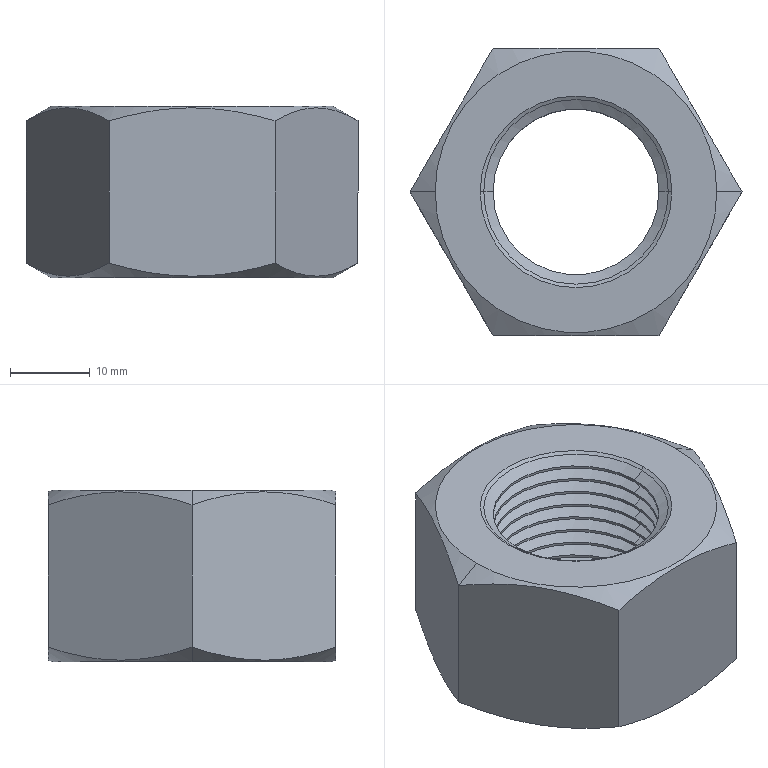Part | SolidWorks | features RevCut 2, Chamfer 1, Extrusion 1, LPattern 1 | 1 solid | 80 faces | box 41.569 x 36 x 21.5 mm | volume 15808 mm3 | cone 52 | cylinder 20 | plane 8 | commonest cylinder face diameters 20.752 x20